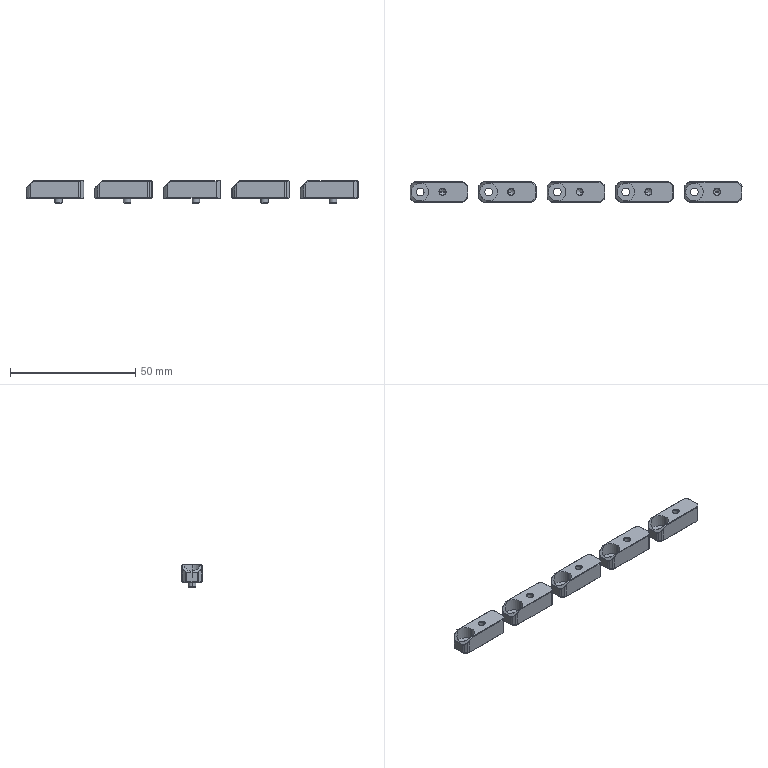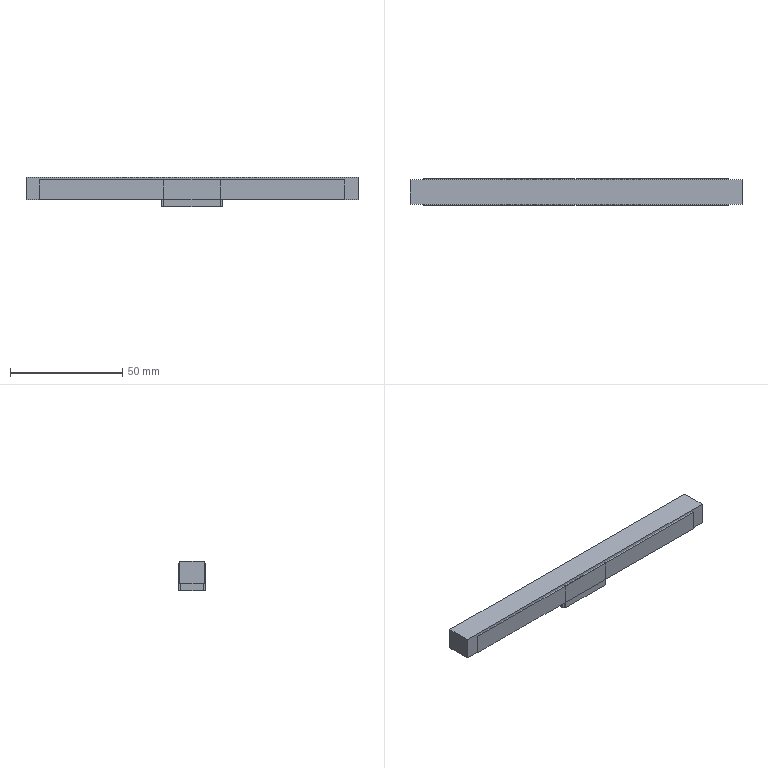CAM job | NX | 3-axis milling, drilling | part box 132.6 x 8 x 8.9 mm | stock box 148 x 12 x 13.1 mm
Tools:
number,name,description,diameter,corner_radius,flute_length,length,flutes
8,钻头D3.2,Drilling Tool,3.2,0.0,35.0,50.0,2
5,钻头2.5,Drilling Tool,2.5,0.0,35.0,50.0,2
6,丝锥M3,Drilling Tool,2.5,0.0,35.0,50.0,2
1,D10J-25L-35L,Milling Tool-5 Parameters,10.0,0.0,25.0,75.0,2
2,4J-10L-25L,Milling Tool-5 Parameters,4.0,0.0,10.0,65.0,2
3,4C-10L-25L,Milling Tool-5 Parameters,4.0,0.0,10.0,65.0,2
4,D8点钻,Drilling Tool,8.0,0.0,10.0,75.0,2
7,R1,Milling Tool-5 Parameters,2.5,1.0,4.0,65.0,2
Operations:
program,operation,operation_type,tool,method,geometry_group,spindle_rpm,surface_speed,feed_per_tooth,feed_cut,feed_plunge,cut_length_mm,path_length_mm,cut_time_min,machine_time_min
A0101,FACE_MILLING,FaceMilling,D10J-25L-35L,METHOD,W1,3500.0,109.0,0.1143,800.0,100.0,158.6,192.6,0.1983,0.2017
A0101,PLANAR_MILL,PlanarMilling,4C-10L-25L,METHOD,W1,4500.0,56.0,0.1667,1500.0,100.0,3904.47,4097.314,2.603,2.622
A0101,HOLE_MILLING,CylinderMilling,4C-10L-25L,METHOD,W1,4500.0,56.0,0.0889,800.0,100.0,542.795,876.395,0.6785,0.7119
A0101,PLANAR_MILL_1_COPY,PlanarMilling,D8点钻,METHOD,W1,3500.0,87.0,0.0857,600.0,100.0,105.858,436.137,0.1764,0.2095
A0101,PLANAR_MILL_1,PlanarMilling,D8点钻,METHOD,W1,3500.0,87.0,0.0857,600.0,100.0,105.858,436.137,0.1764,0.2095
A0101,DRILLING,Operation,D8点钻,METHOD,W1,2500.0,62.0,0.04,200.0,0.0,21.25,205.155,0.1063,0.1246
A0101,DRILLING_COPY,Operation,钻头2.5,METHOD,W1,2500.0,19.0,0.05,250.0,0.0,55.0,272.655,0.22,0.2418
A0101,DRILLING_COPY_COPY,Operation,丝锥M3,METHOD,W1,300.0,2.0,0.0008,0.5,0.0,50.0,262.655,100.0,100.021
A0101,SOLID_PROFILE_3D,PlanarMilling,R1,METHOD,W1,4500.0,28.0,0.0667,600.0,100.0,381.015,665.542,0.635,0.6635
A0101,PLANAR_MILL_COPY,PlanarMilling,4J-10L-25L,METHOD,W1,4000.0,50.0,0.1,800.0,100.0,399.245,644.845,0.4991,0.5236
A0101,PLANAR_MILL_2,PlanarMilling,4J-10L-25L,METHOD,W1,4500.0,56.0,0.0556,500.0,100.0,80.266,412.604,0.1605,0.1938
B0101,ADAPTIVE_MILLING,CavityMilling,D10J-25L-35L,METHOD,W2,5500.0,172.0,0.2273,2500.0,100.0,532.976,666.143,0.2008,0.2141
B0101,PLANAR_MILL_3_COPY,PlanarMilling,4J-10L-25L,METHOD,W2,4500.0,56.0,0.0889,800.0,100.0,146.2,180.2,0.1827,0.1861
B0101,PLANAR_MILL_3,PlanarMilling,4J-10L-25L,METHOD,W2,4500.0,56.0,0.0889,800.0,100.0,695.999,995.599,0.87,0.9
B0101,PLANAR_MILL_4_COPY,PlanarMilling,D8点钻,METHOD,W2,3500.0,87.0,0.1143,800.0,100.0,132.102,426.993,0.1651,0.1946
B0101,PLANAR_MILL_4,PlanarMilling,D8点钻,METHOD,W2,3500.0,87.0,0.1143,800.0,100.0,378.214,604.81,0.4728,0.4954
B0101,DRILLING_1,Operation,D8点钻,METHOD,W2,2500.0,62.0,0.04,200.0,0.0,23.0,212.255,0.115,0.1339
B0101,DRILLING_1_COPY,Operation,钻头D3.2,METHOD,W2,2500.0,62.0,0.04,200.0,0.0,40.0,246.255,0.2,0.2206
SINGLE,FACE_MILLING_COPY,FaceMilling,D10J-25L-35L,METHOD,W1_COPY,3500.0,109.0,0.1143,800.0,100.0,53.0,87.0,0.0662,0.0696
SINGLE,PLANAR_MILL_COPY_1,PlanarMilling,4C-10L-25L,METHOD,W1_COPY,4500.0,56.0,0.1667,1500.0,100.0,637.65,684.05,0.4251,0.4297
SINGLE,PLANAR_MILL_1_COPY_COPY,PlanarMilling,D8点钻,METHOD,W1_COPY,3500.0,87.0,0.0857,600.0,100.0,21.172,62.172,0.0353,0.0394
SINGLE,PLANAR_MILL_1_COPY_1,PlanarMilling,D8点钻,METHOD,W1_COPY,3500.0,87.0,0.0857,600.0,100.0,21.172,62.172,0.0353,0.0394
SINGLE,DRILLING_COPY_1,Operation,D8点钻,METHOD,W1_COPY,2500.0,62.0,0.04,200.0,0.0,4.25,48.9,0.0213,0.0257
SINGLE,HOLE_MILLING_COPY,CylinderMilling,4C-10L-25L,METHOD,W1_COPY,4500.0,56.0,0.0889,800.0,100.0,108.559,153.359,0.1357,0.1402
SINGLE,DRILLING_COPY_COPY_1,Operation,钻头2.5,METHOD,W1_COPY,2500.0,19.0,0.05,250.0,0.0,11.0,62.4,0.044,0.0491
SINGLE,DRILLING_COPY_COPY_COPY,Operation,丝锥M3,METHOD,W1_COPY,300.0,2.0,0.0008,0.5,0.0,10.0,60.4,20.0,20.005
SINGLE,SOLID_PROFILE_3D_COPY,PlanarMilling,R1,METHOD,W1_COPY,4500.0,28.0,0.0667,600.0,100.0,76.253,111.253,0.1271,0.1306
SINGLE,PLANAR_MILL_COPY_COPY,PlanarMilling,4J-10L-25L,METHOD,W1_COPY,4000.0,50.0,0.0375,300.0,100.0,79.849,128.649,0.2662,0.271
SINGLE,PLANAR_MILL_2_COPY,PlanarMilling,4J-10L-25L,METHOD,W1_COPY,4500.0,56.0,0.0167,150.0,100.0,16.053,60.053,0.107,0.1114
单个2,ADAPTIVE_MILLING_COPY,CavityMilling,D10J-25L-35L,METHOD,W2,5500.0,172.0,0.2273,2500.0,100.0,532.184,662.792,0.2007,0.2138
单个2,PLANAR_MILL_3_COPY_COPY,PlanarMilling,4J-10L-25L,METHOD,W2,4500.0,56.0,0.0889,800.0,100.0,16.5,50.5,0.0206,0.024
单个2,PLANAR_MILL_3_COPY_1,PlanarMilling,4J-10L-25L,METHOD,W2,4500.0,56.0,0.0889,800.0,100.0,139.2,177.2,0.174,0.1778
单个2,PLANAR_MILL_4_COPY_COPY,PlanarMilling,D8点钻,METHOD,W2,3500.0,87.0,0.1143,800.0,100.0,26.42,63.42,0.033,0.0367
单个2,PLANAR_MILL_4_COPY_1,PlanarMilling,D8点钻,METHOD,W2,3500.0,87.0,0.1143,800.0,100.0,75.451,116.451,0.0943,0.0984
单个2,DRILLING_1_COPY_1,Operation,D8点钻,METHOD,W2,2500.0,62.0,0.04,200.0,0.0,4.6,53.2,0.023,0.0279
单个2,DRILLING_1_COPY_COPY,Operation,钻头D3.2,METHOD,W2,2500.0,62.0,0.04,200.0,0.0,8.0,60.0,0.04,0.0452